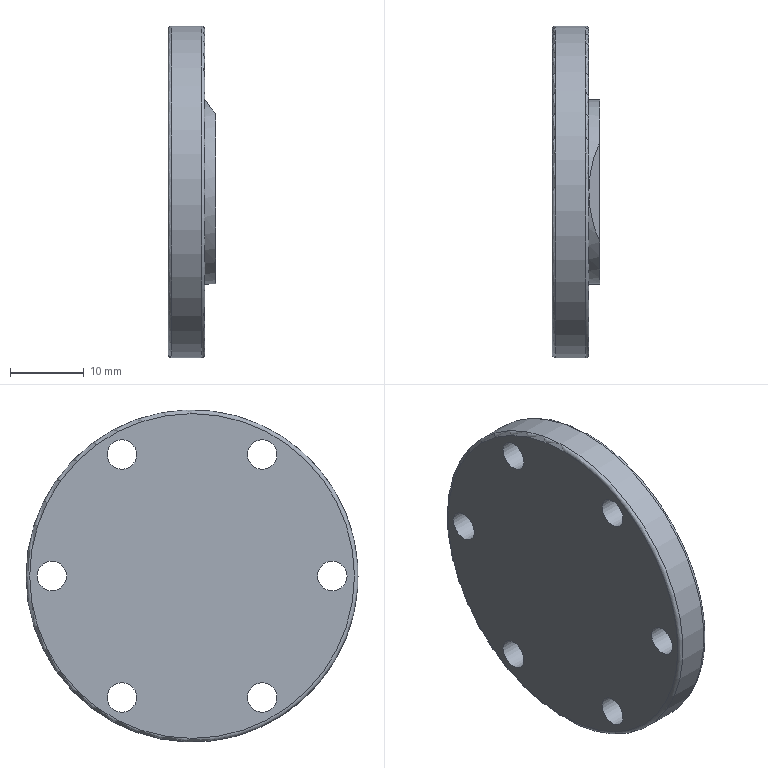Part | STEP file | 1-07 | 1 solid | 15 faces | box 6.5 x 45 x 45 mm | volume 8285 mm3 | cylinder 9 | plane 4 | torus 2 | commonest cylinder face diameters 4 x6 25 x2 45 x1
STEP:
#1=CARTESIAN_POINT('',(0.,0.,0.));
#2=DIRECTION('',(0.,0.,1.));
#3=DIRECTION('',(1.,0.,0.));
#4=AXIS2_PLACEMENT_3D('',#1,#2,#3);
#5=CARTESIAN_POINT('',(0.,21.,0.));
#6=VERTEX_POINT('',#5);
#7=CARTESIAN_POINT('',(0.,19.,0.));
#8=DIRECTION('',(-1.,0.,0.));
#9=DIRECTION('',(0.,1.,0.));
#10=AXIS2_PLACEMENT_3D('',#7,#8,#9);
#11=CIRCLE('',#10,2.);
#12=CARTESIAN_POINT('',(0.,19.,0.));
#13=DIRECTION('',(-1.,0.,0.));
#14=DIRECTION('',(0.,1.,0.));
#15=AXIS2_PLACEMENT_3D('',#12,#13,#14);
#16=CYLINDRICAL_SURFACE('',#15,2.);
#17=CARTESIAN_POINT('',(0.,0.));
#18=DIRECTION('',(1.,0.));
#19=VECTOR('',#18,1.);
#20=LINE('',#17,#19);
#21=(GEOMETRIC_REPRESENTATION_CONTEXT(2)PARAMETRIC_REPRESENTATION_CONTEXT()REPRESENTATION_CONTEXT('',''));
#22=DEFINITIONAL_REPRESENTATION('',(#20),#21);
#23=PCURVE('',#16,#22);
#24=CARTESIAN_POINT('',(0.,-6.029,0.));
#25=DIRECTION('',(1.,0.,0.));
#26=DIRECTION('',(0.,1.,0.));
#27=AXIS2_PLACEMENT_3D('',#24,#25,#26);
#28=PLANE('',#27);
#29=CARTESIAN_POINT('',(27.029,0.));
#30=CARTESIAN_POINT('',(27.029,-3.464));
#31=CARTESIAN_POINT('',(24.029,-1.732));
#32=CARTESIAN_POINT('',(21.029,0.));
#33=CARTESIAN_POINT('',(24.029,1.732));
#34=CARTESIAN_POINT('',(27.029,3.464));
#35=CARTESIAN_POINT('',(27.029,0.));
#36=(BOUNDED_CURVE()B_SPLINE_CURVE(2,(#29,#30,#31,#32,#33,#34,#35),.UNSPECIFIED.,.T.,.F.)B_SPLINE_CURVE_WITH_KNOTS((1,2,2,2,2,1),(-2.094,0.,2.094,4.189,6.283,8.378),.UNSPECIFIED.)CURVE()GEOMETRIC_REPRESENTATION_ITEM()RATIONAL_B_SPLINE_CURVE((1.,0.5,1.,0.5,1.,0.5,1.))REPRESENTATION_ITEM(''));
#37=(GEOMETRIC_REPRESENTATION_CONTEXT(2)PARAMETRIC_REPRESENTATION_CONTEXT()REPRESENTATION_CONTEXT('',''));
#38=DEFINITIONAL_REPRESENTATION('',(#36),#37);
#39=PCURVE('',#28,#38);
#40=SURFACE_CURVE('',#11,(#23,#39),.PCURVE_S1.);
#41=EDGE_CURVE('',#6,#6,#40,.T.);
#42=ORIENTED_EDGE('',*,*,#41,.T.);
#43=CARTESIAN_POINT('',(-5.,21.,0.));
#44=VERTEX_POINT('',#43);
#45=CARTESIAN_POINT('',(0.,21.,0.));
#46=DIRECTION('',(-1.,0.,0.));
#47=VECTOR('',#46,1.);
#48=LINE('',#45,#47);
#49=CARTESIAN_POINT('',(6.283,0.));
#50=DIRECTION('',(0.,1.));
#51=VECTOR('',#50,1.);
#52=LINE('',#49,#51);
#53=(GEOMETRIC_REPRESENTATION_CONTEXT(2)PARAMETRIC_REPRESENTATION_CONTEXT()REPRESENTATION_CONTEXT('',''));
#54=DEFINITIONAL_REPRESENTATION('',(#52),#53);
#55=PCURVE('',#16,#54);
#56=CARTESIAN_POINT('',(0.,0.));
#57=DIRECTION('',(0.,1.));
#58=VECTOR('',#57,1.);
#59=LINE('',#56,#58);
#60=(GEOMETRIC_REPRESENTATION_CONTEXT(2)PARAMETRIC_REPRESENTATION_CONTEXT()REPRESENTATION_CONTEXT('',''));
#61=DEFINITIONAL_REPRESENTATION('',(#59),#60);
#62=PCURVE('',#16,#61);
#63=SEAM_CURVE('',#48,(#55,#62),.PCURVE_S1.);
#64=EDGE_CURVE('',#6,#44,#63,.T.);
#65=ORIENTED_EDGE('',*,*,#64,.T.);
#66=CARTESIAN_POINT('',(-5.,19.,0.));
#67=DIRECTION('',(-1.,0.,0.));
#68=DIRECTION('',(0.,1.,0.));
#69=AXIS2_PLACEMENT_3D('',#66,#67,#68);
#70=CIRCLE('',#69,2.);
#71=CARTESIAN_POINT('',(0.,5.));
#72=DIRECTION('',(1.,0.));
#73=VECTOR('',#72,1.);
#74=LINE('',#71,#73);
#75=(GEOMETRIC_REPRESENTATION_CONTEXT(2)PARAMETRIC_REPRESENTATION_CONTEXT()REPRESENTATION_CONTEXT('',''));
#76=DEFINITIONAL_REPRESENTATION('',(#74),#75);
#77=PCURVE('',#16,#76);
#78=CARTESIAN_POINT('',(-5.,-6.029,0.));
#79=DIRECTION('',(1.,0.,0.));
#80=DIRECTION('',(0.,1.,0.));
#81=AXIS2_PLACEMENT_3D('',#78,#79,#80);
#82=PLANE('',#81);
#83=CARTESIAN_POINT('',(27.029,0.));
#84=CARTESIAN_POINT('',(27.029,-3.464));
#85=CARTESIAN_POINT('',(24.029,-1.732));
#86=CARTESIAN_POINT('',(21.029,0.));
#87=CARTESIAN_POINT('',(24.029,1.732));
#88=CARTESIAN_POINT('',(27.029,3.464));
#89=CARTESIAN_POINT('',(27.029,0.));
#90=(BOUNDED_CURVE()B_SPLINE_CURVE(2,(#83,#84,#85,#86,#87,#88,#89),.UNSPECIFIED.,.T.,.F.)B_SPLINE_CURVE_WITH_KNOTS((1,2,2,2,2,1),(-2.094,0.,2.094,4.189,6.283,8.378),.UNSPECIFIED.)CURVE()GEOMETRIC_REPRESENTATION_ITEM()RATIONAL_B_SPLINE_CURVE((1.,0.5,1.,0.5,1.,0.5,1.))REPRESENTATION_ITEM(''));
#91=(GEOMETRIC_REPRESENTATION_CONTEXT(2)PARAMETRIC_REPRESENTATION_CONTEXT()REPRESENTATION_CONTEXT('',''));
#92=DEFINITIONAL_REPRESENTATION('',(#90),#91);
#93=PCURVE('',#82,#92);
#94=SURFACE_CURVE('',#70,(#77,#93),.PCURVE_S1.);
#95=EDGE_CURVE('',#44,#44,#94,.T.);
#96=ORIENTED_EDGE('',*,*,#95,.F.);
#97=ORIENTED_EDGE('',*,*,#64,.F.);
#98=EDGE_LOOP('',(#42,#65,#96,#97));
#99=FACE_BOUND('',#98,.F.);
#100=ADVANCED_FACE('',(#99),#16,.F.);
#101=CARTESIAN_POINT('',(0.,11.5,16.454));
#102=VERTEX_POINT('',#101);
#103=CARTESIAN_POINT('',(0.,9.5,16.454));
#104=DIRECTION('',(-1.,0.,0.));
#105=DIRECTION('',(0.,1.,0.));
#106=AXIS2_PLACEMENT_3D('',#103,#104,#105);
#107=CIRCLE('',#106,2.);
#108=CARTESIAN_POINT('',(0.,9.5,16.454));
#109=DIRECTION('',(-1.,0.,0.));
#110=DIRECTION('',(0.,1.,0.));
#111=AXIS2_PLACEMENT_3D('',#108,#109,#110);
#112=CYLINDRICAL_SURFACE('',#111,2.);
#113=CARTESIAN_POINT('',(0.,0.));
#114=DIRECTION('',(1.,0.));
#115=VECTOR('',#114,1.);
#116=LINE('',#113,#115);
#117=(GEOMETRIC_REPRESENTATION_CONTEXT(2)PARAMETRIC_REPRESENTATION_CONTEXT()REPRESENTATION_CONTEXT('',''));
#118=DEFINITIONAL_REPRESENTATION('',(#116),#117);
#119=PCURVE('',#112,#118);
#120=CARTESIAN_POINT('',(17.529,16.454));
#121=CARTESIAN_POINT('',(17.529,12.99));
#122=CARTESIAN_POINT('',(14.529,14.722));
#123=CARTESIAN_POINT('',(11.529,16.454));
#124=CARTESIAN_POINT('',(14.529,18.187));
#125=CARTESIAN_POINT('',(17.529,19.919));
#126=CARTESIAN_POINT('',(17.529,16.454));
#127=(BOUNDED_CURVE()B_SPLINE_CURVE(2,(#120,#121,#122,#123,#124,#125,#126),.UNSPECIFIED.,.T.,.F.)B_SPLINE_CURVE_WITH_KNOTS((1,2,2,2,2,1),(-2.094,0.,2.094,4.189,6.283,8.378),.UNSPECIFIED.)CURVE()GEOMETRIC_REPRESENTATION_ITEM()RATIONAL_B_SPLINE_CURVE((1.,0.5,1.,0.5,1.,0.5,1.))REPRESENTATION_ITEM(''));
#128=(GEOMETRIC_REPRESENTATION_CONTEXT(2)PARAMETRIC_REPRESENTATION_CONTEXT()REPRESENTATION_CONTEXT('',''));
#129=DEFINITIONAL_REPRESENTATION('',(#127),#128);
#130=PCURVE('',#28,#129);
#131=SURFACE_CURVE('',#107,(#119,#130),.PCURVE_S1.);
#132=EDGE_CURVE('',#102,#102,#131,.T.);
#133=ORIENTED_EDGE('',*,*,#132,.T.);
#134=CARTESIAN_POINT('',(-5.,11.5,16.454));
#135=VERTEX_POINT('',#134);
#136=CARTESIAN_POINT('',(0.,11.5,16.454));
#137=DIRECTION('',(-1.,0.,0.));
#138=VECTOR('',#137,1.);
#139=LINE('',#136,#138);
#140=CARTESIAN_POINT('',(6.283,0.));
#141=DIRECTION('',(0.,1.));
#142=VECTOR('',#141,1.);
#143=LINE('',#140,#142);
#144=(GEOMETRIC_REPRESENTATION_CONTEXT(2)PARAMETRIC_REPRESENTATION_CONTEXT()REPRESENTATION_CONTEXT('',''));
#145=DEFINITIONAL_REPRESENTATION('',(#143),#144);
#146=PCURVE('',#112,#145);
#147=CARTESIAN_POINT('',(0.,0.));
#148=DIRECTION('',(0.,1.));
#149=VECTOR('',#148,1.);
#150=LINE('',#147,#149);
#151=(GEOMETRIC_REPRESENTATION_CONTEXT(2)PARAMETRIC_REPRESENTATION_CONTEXT()REPRESENTATION_CONTEXT('',''));
#152=DEFINITIONAL_REPRESENTATION('',(#150),#151);
#153=PCURVE('',#112,#152);
#154=SEAM_CURVE('',#139,(#146,#153),.PCURVE_S1.);
#155=EDGE_CURVE('',#102,#135,#154,.T.);
#156=ORIENTED_EDGE('',*,*,#155,.T.);
#157=CARTESIAN_POINT('',(-5.,9.5,16.454));
#158=DIRECTION('',(-1.,0.,0.));
#159=DIRECTION('',(0.,1.,0.));
#160=AXIS2_PLACEMENT_3D('',#157,#158,#159);
#161=CIRCLE('',#160,2.);
#162=CARTESIAN_POINT('',(0.,5.));
#163=DIRECTION('',(1.,0.));
#164=VECTOR('',#163,1.);
#165=LINE('',#162,#164);
#166=(GEOMETRIC_REPRESENTATION_CONTEXT(2)PARAMETRIC_REPRESENTATION_CONTEXT()REPRESENTATION_CONTEXT('',''));
#167=DEFINITIONAL_REPRESENTATION('',(#165),#166);
#168=PCURVE('',#112,#167);
#169=CARTESIAN_POINT('',(17.529,16.454));
#170=CARTESIAN_POINT('',(17.529,12.99));
#171=CARTESIAN_POINT('',(14.529,14.722));
#172=CARTESIAN_POINT('',(11.529,16.454));
#173=CARTESIAN_POINT('',(14.529,18.187));
#174=CARTESIAN_POINT('',(17.529,19.919));
#175=CARTESIAN_POINT('',(17.529,16.454));
#176=(BOUNDED_CURVE()B_SPLINE_CURVE(2,(#169,#170,#171,#172,#173,#174,#175),.UNSPECIFIED.,.T.,.F.)B_SPLINE_CURVE_WITH_KNOTS((1,2,2,2,2,1),(-2.094,0.,2.094,4.189,6.283,8.378),.UNSPECIFIED.)CURVE()GEOMETRIC_REPRESENTATION_ITEM()RATIONAL_B_SPLINE_CURVE((1.,0.5,1.,0.5,1.,0.5,1.))REPRESENTATION_ITEM(''));
#177=(GEOMETRIC_REPRESENTATION_CONTEXT(2)PARAMETRIC_REPRESENTATION_CONTEXT()REPRESENTATION_CONTEXT('',''));
#178=DEFINITIONAL_REPRESENTATION('',(#176),#177);
#179=PCURVE('',#82,#178);
#180=SURFACE_CURVE('',#161,(#168,#179),.PCURVE_S1.);
#181=EDGE_CURVE('',#135,#135,#180,.T.);
#182=ORIENTED_EDGE('',*,*,#181,.F.);
#183=ORIENTED_EDGE('',*,*,#155,.F.);
#184=EDGE_LOOP('',(#133,#156,#182,#183));
#185=FACE_BOUND('',#184,.F.);
#186=ADVANCED_FACE('',(#185),#112,.F.);
#187=CARTESIAN_POINT('',(0.,-7.5,16.454));
#188=VERTEX_POINT('',#187);
#189=CARTESIAN_POINT('',(0.,-9.5,16.454));
#190=DIRECTION('',(-1.,0.,0.));
#191=DIRECTION('',(0.,1.,0.));
#192=AXIS2_PLACEMENT_3D('',#189,#190,#191);
#193=CIRCLE('',#192,2.);
#194=CARTESIAN_POINT('',(0.,-9.5,16.454));
#195=DIRECTION('',(-1.,0.,0.));
#196=DIRECTION('',(0.,1.,0.));
#197=AXIS2_PLACEMENT_3D('',#194,#195,#196);
#198=CYLINDRICAL_SURFACE('',#197,2.);
#199=CARTESIAN_POINT('',(0.,0.));
#200=DIRECTION('',(1.,0.));
#201=VECTOR('',#200,1.);
#202=LINE('',#199,#201);
#203=(GEOMETRIC_REPRESENTATION_CONTEXT(2)PARAMETRIC_REPRESENTATION_CONTEXT()REPRESENTATION_CONTEXT('',''));
#204=DEFINITIONAL_REPRESENTATION('',(#202),#203);
#205=PCURVE('',#198,#204);
#206=CARTESIAN_POINT('',(-1.471,16.454));
#207=CARTESIAN_POINT('',(-1.471,12.99));
#208=CARTESIAN_POINT('',(-4.471,14.722));
#209=CARTESIAN_POINT('',(-7.471,16.454));
#210=CARTESIAN_POINT('',(-4.471,18.187));
#211=CARTESIAN_POINT('',(-1.471,19.919));
#212=CARTESIAN_POINT('',(-1.471,16.454));
#213=(BOUNDED_CURVE()B_SPLINE_CURVE(2,(#206,#207,#208,#209,#210,#211,#212),.UNSPECIFIED.,.T.,.F.)B_SPLINE_CURVE_WITH_KNOTS((1,2,2,2,2,1),(-2.094,0.,2.094,4.189,6.283,8.378),.UNSPECIFIED.)CURVE()GEOMETRIC_REPRESENTATION_ITEM()RATIONAL_B_SPLINE_CURVE((1.,0.5,1.,0.5,1.,0.5,1.))REPRESENTATION_ITEM(''));
#214=(GEOMETRIC_REPRESENTATION_CONTEXT(2)PARAMETRIC_REPRESENTATION_CONTEXT()REPRESENTATION_CONTEXT('',''));
#215=DEFINITIONAL_REPRESENTATION('',(#213),#214);
#216=PCURVE('',#28,#215);
#217=SURFACE_CURVE('',#193,(#205,#216),.PCURVE_S1.);
#218=EDGE_CURVE('',#188,#188,#217,.T.);
#219=ORIENTED_EDGE('',*,*,#218,.T.);
#220=CARTESIAN_POINT('',(-5.,-7.5,16.454));
#221=VERTEX_POINT('',#220);
#222=CARTESIAN_POINT('',(0.,-7.5,16.454));
#223=DIRECTION('',(-1.,0.,0.));
#224=VECTOR('',#223,1.);
#225=LINE('',#222,#224);
#226=CARTESIAN_POINT('',(6.283,0.));
#227=DIRECTION('',(0.,1.));
#228=VECTOR('',#227,1.);
#229=LINE('',#226,#228);
#230=(GEOMETRIC_REPRESENTATION_CONTEXT(2)PARAMETRIC_REPRESENTATION_CONTEXT()REPRESENTATION_CONTEXT('',''));
#231=DEFINITIONAL_REPRESENTATION('',(#229),#230);
#232=PCURVE('',#198,#231);
#233=CARTESIAN_POINT('',(0.,0.));
#234=DIRECTION('',(0.,1.));
#235=VECTOR('',#234,1.);
#236=LINE('',#233,#235);
#237=(GEOMETRIC_REPRESENTATION_CONTEXT(2)PARAMETRIC_REPRESENTATION_CONTEXT()REPRESENTATION_CONTEXT('',''));
#238=DEFINITIONAL_REPRESENTATION('',(#236),#237);
#239=PCURVE('',#198,#238);
#240=SEAM_CURVE('',#225,(#232,#239),.PCURVE_S1.);
#241=EDGE_CURVE('',#188,#221,#240,.T.);
#242=ORIENTED_EDGE('',*,*,#241,.T.);
#243=CARTESIAN_POINT('',(-5.,-9.5,16.454));
#244=DIRECTION('',(-1.,0.,0.));
#245=DIRECTION('',(0.,1.,0.));
#246=AXIS2_PLACEMENT_3D('',#243,#244,#245);
#247=CIRCLE('',#246,2.);
#248=CARTESIAN_POINT('',(0.,5.));
#249=DIRECTION('',(1.,0.));
#250=VECTOR('',#249,1.);
#251=LINE('',#248,#250);
#252=(GEOMETRIC_REPRESENTATION_CONTEXT(2)PARAMETRIC_REPRESENTATION_CONTEXT()REPRESENTATION_CONTEXT('',''));
#253=DEFINITIONAL_REPRESENTATION('',(#251),#252);
#254=PCURVE('',#198,#253);
#255=CARTESIAN_POINT('',(-1.471,16.454));
#256=CARTESIAN_POINT('',(-1.471,12.99));
#257=CARTESIAN_POINT('',(-4.471,14.722));
#258=CARTESIAN_POINT('',(-7.471,16.454));
#259=CARTESIAN_POINT('',(-4.471,18.187));
#260=CARTESIAN_POINT('',(-1.471,19.919));
#261=CARTESIAN_POINT('',(-1.471,16.454));
#262=(BOUNDED_CURVE()B_SPLINE_CURVE(2,(#255,#256,#257,#258,#259,#260,#261),.UNSPECIFIED.,.T.,.F.)B_SPLINE_CURVE_WITH_KNOTS((1,2,2,2,2,1),(-2.094,0.,2.094,4.189,6.283,8.378),.UNSPECIFIED.)CURVE()GEOMETRIC_REPRESENTATION_ITEM()RATIONAL_B_SPLINE_CURVE((1.,0.5,1.,0.5,1.,0.5,1.))REPRESENTATION_ITEM(''));
#263=(GEOMETRIC_REPRESENTATION_CONTEXT(2)PARAMETRIC_REPRESENTATION_CONTEXT()REPRESENTATION_CONTEXT('',''));
#264=DEFINITIONAL_REPRESENTATION('',(#262),#263);
#265=PCURVE('',#82,#264);
#266=SURFACE_CURVE('',#247,(#254,#265),.PCURVE_S1.);
#267=EDGE_CURVE('',#221,#221,#266,.T.);
#268=ORIENTED_EDGE('',*,*,#267,.F.);
#269=ORIENTED_EDGE('',*,*,#241,.F.);
#270=EDGE_LOOP('',(#219,#242,#268,#269));
#271=FACE_BOUND('',#270,.F.);
#272=ADVANCED_FACE('',(#271),#198,.F.);
#273=CARTESIAN_POINT('',(0.,-17.,0.));
#274=VERTEX_POINT('',#273);
#275=CARTESIAN_POINT('',(0.,-19.,0.));
#276=DIRECTION('',(-1.,0.,0.));
#277=DIRECTION('',(0.,1.,0.));
#278=AXIS2_PLACEMENT_3D('',#275,#276,#277);
#279=CIRCLE('',#278,2.);
#280=CARTESIAN_POINT('',(0.,-19.,0.));
#281=DIRECTION('',(-1.,0.,0.));
#282=DIRECTION('',(0.,1.,0.));
#283=AXIS2_PLACEMENT_3D('',#280,#281,#282);
#284=CYLINDRICAL_SURFACE('',#283,2.);
#285=CARTESIAN_POINT('',(0.,0.));
#286=DIRECTION('',(1.,0.));
#287=VECTOR('',#286,1.);
#288=LINE('',#285,#287);
#289=(GEOMETRIC_REPRESENTATION_CONTEXT(2)PARAMETRIC_REPRESENTATION_CONTEXT()REPRESENTATION_CONTEXT('',''));
#290=DEFINITIONAL_REPRESENTATION('',(#288),#289);
#291=PCURVE('',#284,#290);
#292=CARTESIAN_POINT('',(-10.971,0.));
#293=CARTESIAN_POINT('',(-10.971,-3.464));
#294=CARTESIAN_POINT('',(-13.971,-1.732));
#295=CARTESIAN_POINT('',(-16.971,0.));
#296=CARTESIAN_POINT('',(-13.971,1.732));
#297=CARTESIAN_POINT('',(-10.971,3.464));
#298=CARTESIAN_POINT('',(-10.971,0.));
#299=(BOUNDED_CURVE()B_SPLINE_CURVE(2,(#292,#293,#294,#295,#296,#297,#298),.UNSPECIFIED.,.T.,.F.)B_SPLINE_CURVE_WITH_KNOTS((1,2,2,2,2,1),(-2.094,0.,2.094,4.189,6.283,8.378),.UNSPECIFIED.)CURVE()GEOMETRIC_REPRESENTATION_ITEM()RATIONAL_B_SPLINE_CURVE((1.,0.5,1.,0.5,1.,0.5,1.))REPRESENTATION_ITEM(''));
#300=(GEOMETRIC_REPRESENTATION_CONTEXT(2)PARAMETRIC_REPRESENTATION_CONTEXT()REPRESENTATION_CONTEXT('',''));
#301=DEFINITIONAL_REPRESENTATION('',(#299),#300);
#302=PCURVE('',#28,#301);
#303=SURFACE_CURVE('',#279,(#291,#302),.PCURVE_S1.);
#304=EDGE_CURVE('',#274,#274,#303,.T.);
#305=ORIENTED_EDGE('',*,*,#304,.T.);
#306=CARTESIAN_POINT('',(-5.,-17.,0.));
#307=VERTEX_POINT('',#306);
#308=CARTESIAN_POINT('',(0.,-17.,0.));
#309=DIRECTION('',(-1.,0.,0.));
#310=VECTOR('',#309,1.);
#311=LINE('',#308,#310);
#312=CARTESIAN_POINT('',(6.283,0.));
#313=DIRECTION('',(0.,1.));
#314=VECTOR('',#313,1.);
#315=LINE('',#312,#314);
#316=(GEOMETRIC_REPRESENTATION_CONTEXT(2)PARAMETRIC_REPRESENTATION_CONTEXT()REPRESENTATION_CONTEXT('',''));
#317=DEFINITIONAL_REPRESENTATION('',(#315),#316);
#318=PCURVE('',#284,#317);
#319=CARTESIAN_POINT('',(0.,0.));
#320=DIRECTION('',(0.,1.));
#321=VECTOR('',#320,1.);
#322=LINE('',#319,#321);
#323=(GEOMETRIC_REPRESENTATION_CONTEXT(2)PARAMETRIC_REPRESENTATION_CONTEXT()REPRESENTATION_CONTEXT('',''));
#324=DEFINITIONAL_REPRESENTATION('',(#322),#323);
#325=PCURVE('',#284,#324);
#326=SEAM_CURVE('',#311,(#318,#325),.PCURVE_S1.);
#327=EDGE_CURVE('',#274,#307,#326,.T.);
#328=ORIENTED_EDGE('',*,*,#327,.T.);
#329=CARTESIAN_POINT('',(-5.,-19.,0.));
#330=DIRECTION('',(-1.,0.,0.));
#331=DIRECTION('',(0.,1.,0.));
#332=AXIS2_PLACEMENT_3D('',#329,#330,#331);
#333=CIRCLE('',#332,2.);
#334=CARTESIAN_POINT('',(0.,5.));
#335=DIRECTION('',(1.,0.));
#336=VECTOR('',#335,1.);
#337=LINE('',#334,#336);
#338=(GEOMETRIC_REPRESENTATION_CONTEXT(2)PARAMETRIC_REPRESENTATION_CONTEXT()REPRESENTATION_CONTEXT('',''));
#339=DEFINITIONAL_REPRESENTATION('',(#337),#338);
#340=PCURVE('',#284,#339);
#341=CARTESIAN_POINT('',(-10.971,0.));
#342=CARTESIAN_POINT('',(-10.971,-3.464));
#343=CARTESIAN_POINT('',(-13.971,-1.732));
#344=CARTESIAN_POINT('',(-16.971,0.));
#345=CARTESIAN_POINT('',(-13.971,1.732));
#346=CARTESIAN_POINT('',(-10.971,3.464));
#347=CARTESIAN_POINT('',(-10.971,0.));
#348=(BOUNDED_CURVE()B_SPLINE_CURVE(2,(#341,#342,#343,#344,#345,#346,#347),.UNSPECIFIED.,.T.,.F.)B_SPLINE_CURVE_WITH_KNOTS((1,2,2,2,2,1),(-2.094,0.,2.094,4.189,6.283,8.378),.UNSPECIFIED.)CURVE()GEOMETRIC_REPRESENTATION_ITEM()RATIONAL_B_SPLINE_CURVE((1.,0.5,1.,0.5,1.,0.5,1.))REPRESENTATION_ITEM(''));
#349=(GEOMETRIC_REPRESENTATION_CONTEXT(2)PARAMETRIC_REPRESENTATION_CONTEXT()REPRESENTATION_CONTEXT('',''));
#350=DEFINITIONAL_REPRESENTATION('',(#348),#349);
#351=PCURVE('',#82,#350);
#352=SURFACE_CURVE('',#333,(#340,#351),.PCURVE_S1.);
#353=EDGE_CURVE('',#307,#307,#352,.T.);
#354=ORIENTED_EDGE('',*,*,#353,.F.);
#355=ORIENTED_EDGE('',*,*,#327,.F.);
#356=EDGE_LOOP('',(#305,#328,#354,#355));
#357=FACE_BOUND('',#356,.F.);
#358=ADVANCED_FACE('',(#357),#284,.F.);
#359=CARTESIAN_POINT('',(0.,-7.5,-16.454));
#360=VERTEX_POINT('',#359);
#361=CARTESIAN_POINT('',(0.,-9.5,-16.454));
#362=DIRECTION('',(-1.,0.,0.));
#363=DIRECTION('',(0.,1.,0.));
#364=AXIS2_PLACEMENT_3D('',#361,#362,#363);
#365=CIRCLE('',#364,2.);
#366=CARTESIAN_POINT('',(0.,-9.5,-16.454));
#367=DIRECTION('',(-1.,0.,0.));
#368=DIRECTION('',(0.,1.,0.));
#369=AXIS2_PLACEMENT_3D('',#366,#367,#368);
#370=CYLINDRICAL_SURFACE('',#369,2.);
#371=CARTESIAN_POINT('',(0.,0.));
#372=DIRECTION('',(1.,0.));
#373=VECTOR('',#372,1.);
#374=LINE('',#371,#373);
#375=(GEOMETRIC_REPRESENTATION_CONTEXT(2)PARAMETRIC_REPRESENTATION_CONTEXT()REPRESENTATION_CONTEXT('',''));
#376=DEFINITIONAL_REPRESENTATION('',(#374),#375);
#377=PCURVE('',#370,#376);
#378=CARTESIAN_POINT('',(-1.471,-16.454));
#379=CARTESIAN_POINT('',(-1.471,-19.919));
#380=CARTESIAN_POINT('',(-4.471,-18.187));
#381=CARTESIAN_POINT('',(-7.471,-16.454));
#382=CARTESIAN_POINT('',(-4.471,-14.722));
#383=CARTESIAN_POINT('',(-1.471,-12.99));
#384=CARTESIAN_POINT('',(-1.471,-16.454));
#385=(BOUNDED_CURVE()B_SPLINE_CURVE(2,(#378,#379,#380,#381,#382,#383,#384),.UNSPECIFIED.,.T.,.F.)B_SPLINE_CURVE_WITH_KNOTS((1,2,2,2,2,1),(-2.094,0.,2.094,4.189,6.283,8.378),.UNSPECIFIED.)CURVE()GEOMETRIC_REPRESENTATION_ITEM()RATIONAL_B_SPLINE_CURVE((1.,0.5,1.,0.5,1.,0.5,1.))REPRESENTATION_ITEM(''));
#386=(GEOMETRIC_REPRESENTATION_CONTEXT(2)PARAMETRIC_REPRESENTATION_CONTEXT()REPRESENTATION_CONTEXT('',''));
#387=DEFINITIONAL_REPRESENTATION('',(#385),#386);
#388=PCURVE('',#28,#387);
#389=SURFACE_CURVE('',#365,(#377,#388),.PCURVE_S1.);
#390=EDGE_CURVE('',#360,#360,#389,.T.);
#391=ORIENTED_EDGE('',*,*,#390,.T.);
#392=CARTESIAN_POINT('',(-5.,-7.5,-16.454));
#393=VERTEX_POINT('',#392);
#394=CARTESIAN_POINT('',(0.,-7.5,-16.454));
#395=DIRECTION('',(-1.,0.,0.));
#396=VECTOR('',#395,1.);
#397=LINE('',#394,#396);
#398=CARTESIAN_POINT('',(6.283,0.));
#399=DIRECTION('',(0.,1.));
#400=VECTOR('',#399,1.);
#401=LINE('',#398,#400);
#402=(GEOMETRIC_REPRESENTATION_CONTEXT(2)PARAMETRIC_REPRESENTATION_CONTEXT()REPRESENTATION_CONTEXT('',''));
#403=DEFINITIONAL_REPRESENTATION('',(#401),#402);
#404=PCURVE('',#370,#403);
#405=CARTESIAN_POINT('',(0.,0.));
#406=DIRECTION('',(0.,1.));
#407=VECTOR('',#406,1.);
#408=LINE('',#405,#407);
#409=(GEOMETRIC_REPRESENTATION_CONTEXT(2)PARAMETRIC_REPRESENTATION_CONTEXT()REPRESENTATION_CONTEXT('',''));
#410=DEFINITIONAL_REPRESENTATION('',(#408),#409);
#411=PCURVE('',#370,#410);
#412=SEAM_CURVE('',#397,(#404,#411),.PCURVE_S1.);
#413=EDGE_CURVE('',#360,#393,#412,.T.);
#414=ORIENTED_EDGE('',*,*,#413,.T.);
#415=CARTESIAN_POINT('',(-5.,-9.5,-16.454));
#416=DIRECTION('',(-1.,0.,0.));
#417=DIRECTION('',(0.,1.,0.));
#418=AXIS2_PLACEMENT_3D('',#415,#416,#417);
#419=CIRCLE('',#418,2.);
#420=CARTESIAN_POINT('',(0.,5.));
#421=DIRECTION('',(1.,0.));
#422=VECTOR('',#421,1.);
#423=LINE('',#420,#422);
#424=(GEOMETRIC_REPRESENTATION_CONTEXT(2)PARAMETRIC_REPRESENTATION_CONTEXT()REPRESENTATION_CONTEXT('',''));
#425=DEFINITIONAL_REPRESENTATION('',(#423),#424);
#426=PCURVE('',#370,#425);
#427=CARTESIAN_POINT('',(-1.471,-16.454));
#428=CARTESIAN_POINT('',(-1.471,-19.919));
#429=CARTESIAN_POINT('',(-4.471,-18.187));
#430=CARTESIAN_POINT('',(-7.471,-16.454));
#431=CARTESIAN_POINT('',(-4.471,-14.722));
#432=CARTESIAN_POINT('',(-1.471,-12.99));
#433=CARTESIAN_POINT('',(-1.471,-16.454));
#434=(BOUNDED_CURVE()B_SPLINE_CURVE(2,(#427,#428,#429,#430,#431,#432,#433),.UNSPECIFIED.,.T.,.F.)B_SPLINE_CURVE_WITH_KNOTS((1,2,2,2,2,1),(-2.094,0.,2.094,4.189,6.283,8.378),.UNSPECIFIED.)CURVE()GEOMETRIC_REPRESENTATION_ITEM()RATIONAL_B_SPLINE_CURVE((1.,0.5,1.,0.5,1.,0.5,1.))REPRESENTATION_ITEM(''));
#435=(GEOMETRIC_REPRESENTATION_CONTEXT(2)PARAMETRIC_REPRESENTATION_CONTEXT()REPRESENTATION_CONTEXT('',''));
#436=DEFINITIONAL_REPRESENTATION('',(#434),#435);
#437=PCURVE('',#82,#436);
#438=SURFACE_CURVE('',#419,(#426,#437),.PCURVE_S1.);
#439=EDGE_CURVE('',#393,#393,#438,.T.);
#440=ORIENTED_EDGE('',*,*,#439,.F.);
#441=ORIENTED_EDGE('',*,*,#413,.F.);
#442=EDGE_LOOP('',(#391,#414,#440,#441));
#443=FACE_BOUND('',#442,.F.);
#444=ADVANCED_FACE('',(#443),#370,.F.);
#445=CARTESIAN_POINT('',(0.,11.5,-16.454));
#446=VERTEX_POINT('',#445);
#447=CARTESIAN_POINT('',(0.,9.5,-16.454));
#448=DIRECTION('',(-1.,0.,0.));
#449=DIRECTION('',(0.,1.,0.));
#450=AXIS2_PLACEMENT_3D('',#447,#448,#449);
#451=CIRCLE('',#450,2.);
#452=CARTESIAN_POINT('',(0.,9.5,-16.454));
#453=DIRECTION('',(-1.,0.,0.));
#454=DIRECTION('',(0.,1.,0.));
#455=AXIS2_PLACEMENT_3D('',#452,#453,#454);
#456=CYLINDRICAL_SURFACE('',#455,2.);
#457=CARTESIAN_POINT('',(0.,0.));
#458=DIRECTION('',(1.,0.));
#459=VECTOR('',#458,1.);
#460=LINE('',#457,#459);
#461=(GEOMETRIC_REPRESENTATION_CONTEXT(2)PARAMETRIC_REPRESENTATION_CONTEXT()REPRESENTATION_CONTEXT('',''));
#462=DEFINITIONAL_REPRESENTATION('',(#460),#461);
#463=PCURVE('',#456,#462);
#464=CARTESIAN_POINT('',(17.529,-16.454));
#465=CARTESIAN_POINT('',(17.529,-19.919));
#466=CARTESIAN_POINT('',(14.529,-18.187));
#467=CARTESIAN_POINT('',(11.529,-16.454));
#468=CARTESIAN_POINT('',(14.529,-14.722));
#469=CARTESIAN_POINT('',(17.529,-12.99));
#470=CARTESIAN_POINT('',(17.529,-16.454));
#471=(BOUNDED_CURVE()B_SPLINE_CURVE(2,(#464,#465,#466,#467,#468,#469,#470),.UNSPECIFIED.,.T.,.F.)B_SPLINE_CURVE_WITH_KNOTS((1,2,2,2,2,1),(-2.094,0.,2.094,4.189,6.283,8.378),.UNSPECIFIED.)CURVE()GEOMETRIC_REPRESENTATION_ITEM()RATIONAL_B_SPLINE_CURVE((1.,0.5,1.,0.5,1.,0.5,1.))REPRESENTATION_ITEM(''));
#472=(GEOMETRIC_REPRESENTATION_CONTEXT(2)PARAMETRIC_REPRESENTATION_CONTEXT()REPRESENTATION_CONTEXT('',''));
#473=DEFINITIONAL_REPRESENTATION('',(#471),#472);
#474=PCURVE('',#28,#473);
#475=SURFACE_CURVE('',#451,(#463,#474),.PCURVE_S1.);
#476=EDGE_CURVE('',#446,#446,#475,.T.);
#477=ORIENTED_EDGE('',*,*,#476,.T.);
#478=CARTESIAN_POINT('',(-5.,11.5,-16.454));
#479=VERTEX_POINT('',#478);
#480=CARTESIAN_POINT('',(0.,11.5,-16.454));
#481=DIRECTION('',(-1.,0.,0.));
#482=VECTOR('',#481,1.);
#483=LINE('',#480,#482);
#484=CARTESIAN_POINT('',(6.283,0.));
#485=DIRECTION('',(0.,1.));
#486=VECTOR('',#485,1.);
#487=LINE('',#484,#486);
#488=(GEOMETRIC_REPRESENTATION_CONTEXT(2)PARAMETRIC_REPRESENTATION_CONTEXT()REPRESENTATION_CONTEXT('',''));
#489=DEFINITIONAL_REPRESENTATION('',(#487),#488);
#490=PCURVE('',#456,#489);
#491=CARTESIAN_POINT('',(0.,0.));
#492=DIRECTION('',(0.,1.));
#493=VECTOR('',#492,1.);
#494=LINE('',#491,#493);
#495=(GEOMETRIC_REPRESENTATION_CONTEXT(2)PARAMETRIC_REPRESENTATION_CONTEXT()REPRESENTATION_CONTEXT('',''));
#496=DEFINITIONAL_REPRESENTATION('',(#494),#495);
#497=PCURVE('',#456,#496);
#498=SEAM_CURVE('',#483,(#490,#497),.PCURVE_S1.);
#499=EDGE_CURVE('',#446,#479,#498,.T.);
#500=ORIENTED_EDGE('',*,*,#499,.T.);
#501=CARTESIAN_POINT('',(-5.,9.5,-16.454));
#502=DIRECTION('',(-1.,0.,0.));
#503=DIRECTION('',(0.,1.,0.));
#504=AXIS2_PLACEMENT_3D('',#501,#502,#503);
#505=CIRCLE('',#504,2.);
#506=CARTESIAN_POINT('',(0.,5.));
#507=DIRECTION('',(1.,0.));
#508=VECTOR('',#507,1.);
#509=LINE('',#506,#508);
#510=(GEOMETRIC_REPRESENTATION_CONTEXT(2)PARAMETRIC_REPRESENTATION_CONTEXT()REPRESENTATION_CONTEXT('',''));
#511=DEFINITIONAL_REPRESENTATION('',(#509),#510);
#512=PCURVE('',#456,#511);
#513=CARTESIAN_POINT('',(17.529,-16.454));
#514=CARTESIAN_POINT('',(17.529,-19.919));
#515=CARTESIAN_POINT('',(14.529,-18.187));
#516=CARTESIAN_POINT('',(11.529,-16.454));
#517=CARTESIAN_POINT('',(14.529,-14.722));
#518=CARTESIAN_POINT('',(17.529,-12.99));
#519=CARTESIAN_POINT('',(17.529,-16.454));
#520=(BOUNDED_CURVE()B_SPLINE_CURVE(2,(#513,#514,#515,#516,#517,#518,#519),.UNSPECIFIED.,.T.,.F.)B_SPLINE_CURVE_WITH_KNOTS((1,2,2,2,2,1),(-2.094,0.,2.094,4.189,6.283,8.378),.UNSPECIFIED.)CURVE()GEOMETRIC_REPRESENTATION_ITEM()RATIONAL_B_SPLINE_CURVE((1.,0.5,1.,0.5,1.,0.5,1.))REPRESENTATION_ITEM(''));
#521=(GEOMETRIC_REPRESENTATION_CONTEXT(2)PARAMETRIC_REPRESENTATION_CONTEXT()REPRESENTATION_CONTEXT('',''));
#522=DEFINITIONAL_REPRESENTATION('',(#520),#521);
#523=PCURVE('',#82,#522);
#524=SURFACE_CURVE('',#505,(#512,#523),.PCURVE_S1.);
#525=EDGE_CURVE('',#479,#479,#524,.T.);
#526=ORIENTED_EDGE('',*,*,#525,.F.);
#527=ORIENTED_EDGE('',*,*,#499,.F.);
#528=EDGE_LOOP('',(#477,#500,#526,#527));
#529=FACE_BOUND('',#528,.F.);
#530=ADVANCED_FACE('',(#529),#456,.F.);
#531=CARTESIAN_POINT('',(1.5,-6.782,10.5));
#532=VERTEX_POINT('',#531);
#533=CARTESIAN_POINT('',(1.5,12.5,0.));
#534=VERTEX_POINT('',#533);
#535=CARTESIAN_POINT('',(1.5,0.,0.));
#536=DIRECTION('',(1.,0.,0.));
#537=DIRECTION('',(0.,-0.5426,0.84));
#538=AXIS2_PLACEMENT_3D('',#535,#536,#537);
#539=CIRCLE('',#538,12.5);
#540=CARTESIAN_POINT('',(0.,0.,0.));
#541=DIRECTION('',(1.,0.,0.));
#542=DIRECTION('',(0.,1.,0.));
#543=AXIS2_PLACEMENT_3D('',#540,#541,#542);
#544=CYLINDRICAL_SURFACE('',#543,12.5);
#545=CARTESIAN_POINT('',(2.144,1.5));
#546=DIRECTION('',(1.,0.));
#547=VECTOR('',#546,1.);
#548=LINE('',#545,#547);
#549=(GEOMETRIC_REPRESENTATION_CONTEXT(2)PARAMETRIC_REPRESENTATION_CONTEXT()REPRESENTATION_CONTEXT('',''));
#550=DEFINITIONAL_REPRESENTATION('',(#548),#549);
#551=PCURVE('',#544,#550);
#552=CARTESIAN_POINT('',(1.5,-3.349,0.));
#553=DIRECTION('',(1.,0.,0.));
#554=DIRECTION('',(0.,1.,0.));
#555=AXIS2_PLACEMENT_3D('',#552,#553,#554);
#556=PLANE('',#555);
#557=CARTESIAN_POINT('',(3.349,0.));
#558=DIRECTION('',(-0.5426,0.84));
#559=AXIS2_PLACEMENT_2D('',#557,#558);
#560=CIRCLE('',#559,12.5);
#561=(GEOMETRIC_REPRESENTATION_CONTEXT(2)PARAMETRIC_REPRESENTATION_CONTEXT()REPRESENTATION_CONTEXT('',''));
#562=DEFINITIONAL_REPRESENTATION('',(#560),#561);
#563=PCURVE('',#556,#562);
#564=SURFACE_CURVE('',#539,(#551,#563),.PCURVE_S1.);
#565=EDGE_CURVE('',#532,#534,#564,.T.);
#566=ORIENTED_EDGE('',*,*,#565,.F.);
#567=CARTESIAN_POINT('',(0.,0.,12.5));
#568=VERTEX_POINT('',#567);
#569=CARTESIAN_POINT('',(9.375,0.,0.));
#570=DIRECTION('',(0.8,0.,0.6));
#571=DIRECTION('',(-0.6,0.,0.8));
#572=AXIS2_PLACEMENT_3D('',#569,#570,#571);
#573=ELLIPSE('',#572,15.625,12.5);
#574=CARTESIAN_POINT('',(1.571,0.));
#575=CARTESIAN_POINT('',(1.579,-0.000000361));
#576=CARTESIAN_POINT('',(1.597,0.002124));
#577=CARTESIAN_POINT('',(1.623,0.01168));
#578=CARTESIAN_POINT('',(1.649,0.0276));
#579=CARTESIAN_POINT('',(1.675,0.04987));
#580=CARTESIAN_POINT('',(1.701,0.07847));
#581=CARTESIAN_POINT('',(1.727,0.1134));
#582=CARTESIAN_POINT('',(1.753,0.1546));
#583=CARTESIAN_POINT('',(1.779,0.2021));
#584=CARTESIAN_POINT('',(1.805,0.2558));
#585=CARTESIAN_POINT('',(1.831,0.3157));
#586=CARTESIAN_POINT('',(1.858,0.3818));
#587=CARTESIAN_POINT('',(1.884,0.454));
#588=CARTESIAN_POINT('',(1.91,0.5322));
#589=CARTESIAN_POINT('',(1.936,0.6165));
#590=CARTESIAN_POINT('',(1.962,0.7067));
#591=CARTESIAN_POINT('',(1.988,0.8028));
#592=CARTESIAN_POINT('',(2.014,0.9047));
#593=CARTESIAN_POINT('',(2.04,1.012));
#594=CARTESIAN_POINT('',(2.066,1.126));
#595=CARTESIAN_POINT('',(2.092,1.245));
#596=CARTESIAN_POINT('',(2.118,1.369));
#597=CARTESIAN_POINT('',(2.136,1.456));
#598=CARTESIAN_POINT('',(2.144,1.5));
#599=B_SPLINE_CURVE_WITH_KNOTS('',3,(#574,#575,#576,#577,#578,#579,#580,#581,#582,#583,#584,#585,#586,#587,#588,#589,#590,#591,#592,#593,#594,#595,#596,#597,#598),.UNSPECIFIED.,.F.,.F.,(4,1,1,1,1,1,1,1,1,1,1,1,1,1,1,1,1,1,1,1,1,1,4),(0.,0.02607,0.05214,0.07821,0.1043,0.1303,0.1564,0.1825,0.2086,0.2346,0.2607,0.2868,0.3128,0.3389,0.365,0.391,0.4171,0.4432,0.4692,0.4953,0.5214,0.5474,0.5735),.UNSPECIFIED.);
#600=(GEOMETRIC_REPRESENTATION_CONTEXT(2)PARAMETRIC_REPRESENTATION_CONTEXT()REPRESENTATION_CONTEXT('',''));
#601=DEFINITIONAL_REPRESENTATION('',(#599),#600);
#602=PCURVE('',#544,#601);
#603=CARTESIAN_POINT('',(0.75,0.,11.5));
#604=DIRECTION('',(-0.8,0.,-0.6));
#605=DIRECTION('',(0.6,0.,-0.8));
#606=AXIS2_PLACEMENT_3D('',#603,#604,#605);
#607=PLANE('',#606);
#608=CARTESIAN_POINT('',(-1.25,0.));
#609=CARTESIAN_POINT('',(-1.25,21.651));
#610=CARTESIAN_POINT('',(22.187,10.825));
#611=CARTESIAN_POINT('',(45.625,0.));
#612=CARTESIAN_POINT('',(22.187,-10.825));
#613=CARTESIAN_POINT('',(-1.25,-21.651));
#614=CARTESIAN_POINT('',(-1.25,0.));
#615=(BOUNDED_CURVE()B_SPLINE_CURVE(2,(#608,#609,#610,#611,#612,#613,#614),.UNSPECIFIED.,.T.,.F.)B_SPLINE_CURVE_WITH_KNOTS((1,2,2,2,2,1),(-2.094,0.,2.094,4.189,6.283,8.378),.UNSPECIFIED.)CURVE()GEOMETRIC_REPRESENTATION_ITEM()RATIONAL_B_SPLINE_CURVE((1.,0.5,1.,0.5,1.,0.5,1.))REPRESENTATION_ITEM(''));
#616=(GEOMETRIC_REPRESENTATION_CONTEXT(2)PARAMETRIC_REPRESENTATION_CONTEXT()REPRESENTATION_CONTEXT('',''));
#617=DEFINITIONAL_REPRESENTATION('',(#615),#616);
#618=PCURVE('',#607,#617);
#619=SURFACE_CURVE('',#573,(#602,#618),.PCURVE_S1.);
#620=EDGE_CURVE('',#568,#532,#619,.T.);
#621=ORIENTED_EDGE('',*,*,#620,.F.);
#622=CARTESIAN_POINT('',(0.,12.5,0.));
#623=VERTEX_POINT('',#622);
#624=CARTESIAN_POINT('',(0.,0.,0.));
#625=DIRECTION('',(1.,0.,0.));
#626=DIRECTION('',(0.,0.,1.));
#627=AXIS2_PLACEMENT_3D('',#624,#625,#626);
#628=CIRCLE('',#627,12.5);
#629=CARTESIAN_POINT('',(1.571,0.));
#630=DIRECTION('',(1.,0.));
#631=VECTOR('',#630,1.);
#632=LINE('',#629,#631);
#633=(GEOMETRIC_REPRESENTATION_CONTEXT(2)PARAMETRIC_REPRESENTATION_CONTEXT()REPRESENTATION_CONTEXT('',''));
#634=DEFINITIONAL_REPRESENTATION('',(#632),#633);
#635=PCURVE('',#544,#634);
#636=CARTESIAN_POINT('',(6.029,0.));
#637=DIRECTION('',(0.,1.));
#638=AXIS2_PLACEMENT_2D('',#636,#637);
#639=CIRCLE('',#638,12.5);
#640=(GEOMETRIC_REPRESENTATION_CONTEXT(2)PARAMETRIC_REPRESENTATION_CONTEXT()REPRESENTATION_CONTEXT('',''));
#641=DEFINITIONAL_REPRESENTATION('',(#639),#640);
#642=PCURVE('',#28,#641);
#643=SURFACE_CURVE('',#628,(#635,#642),.PCURVE_S1.);
#644=EDGE_CURVE('',#568,#623,#643,.T.);
#645=ORIENTED_EDGE('',*,*,#644,.T.);
#646=CARTESIAN_POINT('',(0.,12.5,0.));
#647=DIRECTION('',(1.,0.,0.));
#648=VECTOR('',#647,1.);
#649=LINE('',#646,#648);
#650=CARTESIAN_POINT('',(6.283,0.));
#651=DIRECTION('',(0.,1.));
#652=VECTOR('',#651,1.);
#653=LINE('',#650,#652);
#654=(GEOMETRIC_REPRESENTATION_CONTEXT(2)PARAMETRIC_REPRESENTATION_CONTEXT()REPRESENTATION_CONTEXT('',''));
#655=DEFINITIONAL_REPRESENTATION('',(#653),#654);
#656=PCURVE('',#544,#655);
#657=CARTESIAN_POINT('',(0.,0.,0.));
#658=DIRECTION('',(1.,0.,0.));
#659=DIRECTION('',(0.,1.,0.));
#660=AXIS2_PLACEMENT_3D('',#657,#658,#659);
#661=CYLINDRICAL_SURFACE('',#660,12.5);
#662=CARTESIAN_POINT('',(0.,0.));
#663=DIRECTION('',(0.,1.));
#664=VECTOR('',#663,1.);
#665=LINE('',#662,#664);
#666=(GEOMETRIC_REPRESENTATION_CONTEXT(2)PARAMETRIC_REPRESENTATION_CONTEXT()REPRESENTATION_CONTEXT('',''));
#667=DEFINITIONAL_REPRESENTATION('',(#665),#666);
#668=PCURVE('',#661,#667);
#669=SURFACE_CURVE('',#649,(#656,#668),.PCURVE_S1.);
#670=EDGE_CURVE('',#623,#534,#669,.T.);
#671=ORIENTED_EDGE('',*,*,#670,.T.);
#672=EDGE_LOOP('',(#566,#621,#645,#671));
#673=FACE_BOUND('',#672,.T.);
#674=ADVANCED_FACE('',(#673),#544,.T.);
#675=CARTESIAN_POINT('',(0.,0.,0.));
#676=DIRECTION('',(1.,0.,0.));
#677=DIRECTION('',(0.,1.,0.));
#678=AXIS2_PLACEMENT_3D('',#675,#676,#677);
#679=CIRCLE('',#678,12.5);
#680=CARTESIAN_POINT('',(0.,0.));
#681=DIRECTION('',(1.,0.));
#682=VECTOR('',#681,1.);
#683=LINE('',#680,#682);
#684=(GEOMETRIC_REPRESENTATION_CONTEXT(2)PARAMETRIC_REPRESENTATION_CONTEXT()REPRESENTATION_CONTEXT('',''));
#685=DEFINITIONAL_REPRESENTATION('',(#683),#684);
#686=PCURVE('',#661,#685);
#687=CARTESIAN_POINT('',(6.029,0.));
#688=DIRECTION('',(1.,0.));
#689=AXIS2_PLACEMENT_2D('',#687,#688);
#690=CIRCLE('',#689,12.5);
#691=(GEOMETRIC_REPRESENTATION_CONTEXT(2)PARAMETRIC_REPRESENTATION_CONTEXT()REPRESENTATION_CONTEXT('',''));
#692=DEFINITIONAL_REPRESENTATION('',(#690),#691);
#693=PCURVE('',#28,#692);
#694=SURFACE_CURVE('',#679,(#686,#693),.PCURVE_S1.);
#695=EDGE_CURVE('',#623,#568,#694,.T.);
#696=ORIENTED_EDGE('',*,*,#695,.T.);
#697=CARTESIAN_POINT('',(1.5,6.782,10.5));
#698=VERTEX_POINT('',#697);
#699=CARTESIAN_POINT('',(9.375,0.,0.));
#700=DIRECTION('',(0.8,0.,0.6));
#701=DIRECTION('',(-0.6,0.,0.8));
#702=AXIS2_PLACEMENT_3D('',#699,#700,#701);
#703=ELLIPSE('',#702,15.625,12.5);
#704=CARTESIAN_POINT('',(0.9973,1.5));
#705=CARTESIAN_POINT('',(1.006,1.456));
#706=CARTESIAN_POINT('',(1.023,1.369));
#707=CARTESIAN_POINT('',(1.049,1.245));
#708=CARTESIAN_POINT('',(1.075,1.126));
#709=CARTESIAN_POINT('',(1.102,1.012));
#710=CARTESIAN_POINT('',(1.128,0.9047));
#711=CARTESIAN_POINT('',(1.154,0.8028));
#712=CARTESIAN_POINT('',(1.18,0.7067));
#713=CARTESIAN_POINT('',(1.206,0.6165));
#714=CARTESIAN_POINT('',(1.232,0.5322));
#715=CARTESIAN_POINT('',(1.258,0.454));
#716=CARTESIAN_POINT('',(1.284,0.3818));
#717=CARTESIAN_POINT('',(1.31,0.3157));
#718=CARTESIAN_POINT('',(1.336,0.2558));
#719=CARTESIAN_POINT('',(1.362,0.2021));
#720=CARTESIAN_POINT('',(1.388,0.1546));
#721=CARTESIAN_POINT('',(1.414,0.1134));
#722=CARTESIAN_POINT('',(1.44,0.07847));
#723=CARTESIAN_POINT('',(1.467,0.04987));
#724=CARTESIAN_POINT('',(1.493,0.0276));
#725=CARTESIAN_POINT('',(1.519,0.01168));
#726=CARTESIAN_POINT('',(1.545,0.002124));
#727=CARTESIAN_POINT('',(1.562,-0.000000361));
#728=CARTESIAN_POINT('',(1.571,0.));
#729=B_SPLINE_CURVE_WITH_KNOTS('',3,(#704,#705,#706,#707,#708,#709,#710,#711,#712,#713,#714,#715,#716,#717,#718,#719,#720,#721,#722,#723,#724,#725,#726,#727,#728),.UNSPECIFIED.,.F.,.F.,(4,1,1,1,1,1,1,1,1,1,1,1,1,1,1,1,1,1,1,1,1,1,4),(5.71,5.736,5.762,5.788,5.814,5.84,5.866,5.892,5.918,5.944,5.97,5.996,6.022,6.049,6.075,6.101,6.127,6.153,6.179,6.205,6.231,6.257,6.283),.QUASI_UNIFORM_KNOTS.);
#730=(GEOMETRIC_REPRESENTATION_CONTEXT(2)PARAMETRIC_REPRESENTATION_CONTEXT()REPRESENTATION_CONTEXT('',''));
#731=DEFINITIONAL_REPRESENTATION('',(#729),#730);
#732=PCURVE('',#661,#731);
#733=CARTESIAN_POINT('',(-1.25,0.));
#734=CARTESIAN_POINT('',(-1.25,21.651));
#735=CARTESIAN_POINT('',(22.188,10.825));
#736=CARTESIAN_POINT('',(45.625,0.));
#737=CARTESIAN_POINT('',(22.188,-10.825));
#738=CARTESIAN_POINT('',(-1.25,-21.651));
#739=CARTESIAN_POINT('',(-1.25,0.));
#740=(BOUNDED_CURVE()B_SPLINE_CURVE(2,(#733,#734,#735,#736,#737,#738,#739),.UNSPECIFIED.,.T.,.F.)B_SPLINE_CURVE_WITH_KNOTS((1,2,2,2,2,1),(-2.094,0.,2.094,4.189,6.283,8.378),.UNSPECIFIED.)CURVE()GEOMETRIC_REPRESENTATION_ITEM()RATIONAL_B_SPLINE_CURVE((1.,0.5,1.,0.5,1.,0.5,1.))REPRESENTATION_ITEM(''));
#741=(GEOMETRIC_REPRESENTATION_CONTEXT(2)PARAMETRIC_REPRESENTATION_CONTEXT()REPRESENTATION_CONTEXT('',''));
#742=DEFINITIONAL_REPRESENTATION('',(#740),#741);
#743=PCURVE('',#607,#742);
#744=SURFACE_CURVE('',#703,(#732,#743),.PCURVE_S1.);
#745=EDGE_CURVE('',#698,#568,#744,.T.);
#746=ORIENTED_EDGE('',*,*,#745,.F.);
#747=CARTESIAN_POINT('',(1.5,0.,0.));
#748=DIRECTION('',(1.,0.,0.));
#749=DIRECTION('',(0.,1.,0.));
#750=AXIS2_PLACEMENT_3D('',#747,#748,#749);
#751=CIRCLE('',#750,12.5);
#752=CARTESIAN_POINT('',(0.,1.5));
#753=DIRECTION('',(1.,0.));
#754=VECTOR('',#753,1.);
#755=LINE('',#752,#754);
#756=(GEOMETRIC_REPRESENTATION_CONTEXT(2)PARAMETRIC_REPRESENTATION_CONTEXT()REPRESENTATION_CONTEXT('',''));
#757=DEFINITIONAL_REPRESENTATION('',(#755),#756);
#758=PCURVE('',#661,#757);
#759=CARTESIAN_POINT('',(3.349,0.));
#760=DIRECTION('',(1.,0.));
#761=AXIS2_PLACEMENT_2D('',#759,#760);
#762=CIRCLE('',#761,12.5);
#763=(GEOMETRIC_REPRESENTATION_CONTEXT(2)PARAMETRIC_REPRESENTATION_CONTEXT()REPRESENTATION_CONTEXT('',''));
#764=DEFINITIONAL_REPRESENTATION('',(#762),#763);
#765=PCURVE('',#556,#764);
#766=SURFACE_CURVE('',#751,(#758,#765),.PCURVE_S1.);
#767=EDGE_CURVE('',#534,#698,#766,.T.);
#768=ORIENTED_EDGE('',*,*,#767,.F.);
#769=ORIENTED_EDGE('',*,*,#670,.F.);
#770=EDGE_LOOP('',(#696,#746,#768,#769));
#771=FACE_BOUND('',#770,.T.);
#772=ADVANCED_FACE('',(#771),#661,.T.);
#773=ORIENTED_EDGE('',*,*,#767,.T.);
#774=CARTESIAN_POINT('',(1.5,6.782,10.5));
#775=DIRECTION('',(0.,-1.,0.));
#776=VECTOR('',#775,1.);
#777=LINE('',#774,#776);
#778=CARTESIAN_POINT('',(10.132,10.5));
#779=DIRECTION('',(-1.,0.));
#780=VECTOR('',#779,1.);
#781=LINE('',#778,#780);
#782=(GEOMETRIC_REPRESENTATION_CONTEXT(2)PARAMETRIC_REPRESENTATION_CONTEXT()REPRESENTATION_CONTEXT('',''));
#783=DEFINITIONAL_REPRESENTATION('',(#781),#782);
#784=PCURVE('',#556,#783);
#785=CARTESIAN_POINT('',(1.25,-6.782));
#786=DIRECTION('',(0.,1.));
#787=VECTOR('',#786,1.);
#788=LINE('',#785,#787);
#789=(GEOMETRIC_REPRESENTATION_CONTEXT(2)PARAMETRIC_REPRESENTATION_CONTEXT()REPRESENTATION_CONTEXT('',''));
#790=DEFINITIONAL_REPRESENTATION('',(#788),#789);
#791=PCURVE('',#607,#790);
#792=SURFACE_CURVE('',#777,(#784,#791),.PCURVE_S1.);
#793=EDGE_CURVE('',#698,#532,#792,.T.);
#794=ORIENTED_EDGE('',*,*,#793,.T.);
#795=ORIENTED_EDGE('',*,*,#565,.T.);
#796=EDGE_LOOP('',(#773,#794,#795));
#797=FACE_BOUND('',#796,.T.);
#798=ADVANCED_FACE('',(#797),#556,.T.);
#799=ORIENTED_EDGE('',*,*,#793,.T.);
#800=ORIENTED_EDGE('',*,*,#620,.F.);
#801=ORIENTED_EDGE('',*,*,#745,.F.);
#802=EDGE_LOOP('',(#799,#800,#801));
#803=FACE_BOUND('',#802,.F.);
#804=ADVANCED_FACE('',(#803),#607,.F.);
#805=CARTESIAN_POINT('',(-5.,22.,0.));
#806=VERTEX_POINT('',#805);
#807=CARTESIAN_POINT('',(-5.,0.,0.));
#808=DIRECTION('',(1.,0.,0.));
#809=DIRECTION('',(0.,1.,0.));
#810=AXIS2_PLACEMENT_3D('',#807,#808,#809);
#811=CIRCLE('',#810,22.);
#812=CARTESIAN_POINT('',(6.029,0.));
#813=DIRECTION('',(1.,0.));
#814=AXIS2_PLACEMENT_2D('',#812,#813);
#815=CIRCLE('',#814,22.);
#816=(GEOMETRIC_REPRESENTATION_CONTEXT(2)PARAMETRIC_REPRESENTATION_CONTEXT()REPRESENTATION_CONTEXT('',''));
#817=DEFINITIONAL_REPRESENTATION('',(#815),#816);
#818=PCURVE('',#82,#817);
#819=CARTESIAN_POINT('',(-4.5,0.,0.));
#820=DIRECTION('',(-1.,0.,0.));
#821=DIRECTION('',(0.,1.,0.));
#822=AXIS2_PLACEMENT_3D('',#819,#820,#821);
#823=TOROIDAL_SURFACE('',#822,22.,0.5);
#824=CARTESIAN_POINT('',(6.283,1.571));
#825=DIRECTION('',(-1.,0.));
#826=VECTOR('',#825,1.);
#827=LINE('',#824,#826);
#828=(GEOMETRIC_REPRESENTATION_CONTEXT(2)PARAMETRIC_REPRESENTATION_CONTEXT()REPRESENTATION_CONTEXT('',''));
#829=DEFINITIONAL_REPRESENTATION('',(#827),#828);
#830=PCURVE('',#823,#829);
#831=SURFACE_CURVE('',#811,(#818,#830),.PCURVE_S1.);
#832=EDGE_CURVE('',#806,#806,#831,.T.);
#833=ORIENTED_EDGE('',*,*,#832,.T.);
#834=EDGE_LOOP('',(#833));
#835=FACE_BOUND('',#834,.F.);
#836=ORIENTED_EDGE('',*,*,#525,.T.);
#837=EDGE_LOOP('',(#836));
#838=FACE_BOUND('',#837,.F.);
#839=ORIENTED_EDGE('',*,*,#439,.T.);
#840=EDGE_LOOP('',(#839));
#841=FACE_BOUND('',#840,.F.);
#842=ORIENTED_EDGE('',*,*,#353,.T.);
#843=EDGE_LOOP('',(#842));
#844=FACE_BOUND('',#843,.F.);
#845=ORIENTED_EDGE('',*,*,#267,.T.);
#846=EDGE_LOOP('',(#845));
#847=FACE_BOUND('',#846,.F.);
#848=ORIENTED_EDGE('',*,*,#181,.T.);
#849=EDGE_LOOP('',(#848));
#850=FACE_BOUND('',#849,.F.);
#851=ORIENTED_EDGE('',*,*,#95,.T.);
#852=EDGE_LOOP('',(#851));
#853=FACE_BOUND('',#852,.F.);
#854=ADVANCED_FACE('',(#835,#838,#841,#844,#847,#850,#853),#82,.F.);
#855=CARTESIAN_POINT('',(-0.5,22.5,0.));
#856=VERTEX_POINT('',#855);
#857=CARTESIAN_POINT('',(-0.5,0.,0.));
#858=DIRECTION('',(1.,0.,0.));
#859=DIRECTION('',(0.,1.,0.));
#860=AXIS2_PLACEMENT_3D('',#857,#858,#859);
#861=CIRCLE('',#860,22.5);
#862=CARTESIAN_POINT('',(0.,0.,0.));
#863=DIRECTION('',(-1.,0.,0.));
#864=DIRECTION('',(0.,1.,0.));
#865=AXIS2_PLACEMENT_3D('',#862,#863,#864);
#866=CYLINDRICAL_SURFACE('',#865,22.5);
#867=CARTESIAN_POINT('',(6.283,0.5));
#868=DIRECTION('',(-1.,0.));
#869=VECTOR('',#868,1.);
#870=LINE('',#867,#869);
#871=(GEOMETRIC_REPRESENTATION_CONTEXT(2)PARAMETRIC_REPRESENTATION_CONTEXT()REPRESENTATION_CONTEXT('',''));
#872=DEFINITIONAL_REPRESENTATION('',(#870),#871);
#873=PCURVE('',#866,#872);
#874=CARTESIAN_POINT('',(-0.5,0.,0.));
#875=DIRECTION('',(-1.,0.,0.));
#876=DIRECTION('',(0.,1.,0.));
#877=AXIS2_PLACEMENT_3D('',#874,#875,#876);
#878=TOROIDAL_SURFACE('',#877,22.,0.5);
#879=CARTESIAN_POINT('',(6.283,6.283));
#880=DIRECTION('',(-1.,0.));
#881=VECTOR('',#880,1.);
#882=LINE('',#879,#881);
#883=(GEOMETRIC_REPRESENTATION_CONTEXT(2)PARAMETRIC_REPRESENTATION_CONTEXT()REPRESENTATION_CONTEXT('',''));
#884=DEFINITIONAL_REPRESENTATION('',(#882),#883);
#885=PCURVE('',#878,#884);
#886=SURFACE_CURVE('',#861,(#873,#885),.PCURVE_S1.);
#887=EDGE_CURVE('',#856,#856,#886,.T.);
#888=ORIENTED_EDGE('',*,*,#887,.F.);
#889=CARTESIAN_POINT('',(-4.5,22.5,0.));
#890=VERTEX_POINT('',#889);
#891=CARTESIAN_POINT('',(-0.5,22.5,0.));
#892=DIRECTION('',(-1.,0.,0.));
#893=VECTOR('',#892,1.);
#894=LINE('',#891,#893);
#895=CARTESIAN_POINT('',(6.283,0.5));
#896=DIRECTION('',(0.,1.));
#897=VECTOR('',#896,1.);
#898=LINE('',#895,#897);
#899=(GEOMETRIC_REPRESENTATION_CONTEXT(2)PARAMETRIC_REPRESENTATION_CONTEXT()REPRESENTATION_CONTEXT('',''));
#900=DEFINITIONAL_REPRESENTATION('',(#898),#899);
#901=PCURVE('',#866,#900);
#902=CARTESIAN_POINT('',(0.,0.5));
#903=DIRECTION('',(0.,1.));
#904=VECTOR('',#903,1.);
#905=LINE('',#902,#904);
#906=(GEOMETRIC_REPRESENTATION_CONTEXT(2)PARAMETRIC_REPRESENTATION_CONTEXT()REPRESENTATION_CONTEXT('',''));
#907=DEFINITIONAL_REPRESENTATION('',(#905),#906);
#908=PCURVE('',#866,#907);
#909=SEAM_CURVE('',#894,(#901,#908),.PCURVE_S1.);
#910=EDGE_CURVE('',#856,#890,#909,.T.);
#911=ORIENTED_EDGE('',*,*,#910,.T.);
#912=CARTESIAN_POINT('',(-4.5,0.,0.));
#913=DIRECTION('',(1.,0.,0.));
#914=DIRECTION('',(0.,1.,0.));
#915=AXIS2_PLACEMENT_3D('',#912,#913,#914);
#916=CIRCLE('',#915,22.5);
#917=CARTESIAN_POINT('',(6.283,4.5));
#918=DIRECTION('',(-1.,0.));
#919=VECTOR('',#918,1.);
#920=LINE('',#917,#919);
#921=(GEOMETRIC_REPRESENTATION_CONTEXT(2)PARAMETRIC_REPRESENTATION_CONTEXT()REPRESENTATION_CONTEXT('',''));
#922=DEFINITIONAL_REPRESENTATION('',(#920),#921);
#923=PCURVE('',#866,#922);
#924=CARTESIAN_POINT('',(6.283,0.));
#925=DIRECTION('',(-1.,0.));
#926=VECTOR('',#925,1.);
#927=LINE('',#924,#926);
#928=(GEOMETRIC_REPRESENTATION_CONTEXT(2)PARAMETRIC_REPRESENTATION_CONTEXT()REPRESENTATION_CONTEXT('',''));
#929=DEFINITIONAL_REPRESENTATION('',(#927),#928);
#930=PCURVE('',#823,#929);
#931=SURFACE_CURVE('',#916,(#923,#930),.PCURVE_S1.);
#932=EDGE_CURVE('',#890,#890,#931,.T.);
#933=ORIENTED_EDGE('',*,*,#932,.T.);
#934=ORIENTED_EDGE('',*,*,#910,.F.);
#935=EDGE_LOOP('',(#888,#911,#933,#934));
#936=FACE_BOUND('',#935,.T.);
#937=ADVANCED_FACE('',(#936),#866,.T.);
#938=CARTESIAN_POINT('',(0.,22.,0.));
#939=VERTEX_POINT('',#938);
#940=CARTESIAN_POINT('',(0.,0.,0.));
#941=DIRECTION('',(1.,0.,0.));
#942=DIRECTION('',(0.,1.,0.));
#943=AXIS2_PLACEMENT_3D('',#940,#941,#942);
#944=CIRCLE('',#943,22.);
#945=CARTESIAN_POINT('',(6.029,0.));
#946=DIRECTION('',(1.,0.));
#947=AXIS2_PLACEMENT_2D('',#945,#946);
#948=CIRCLE('',#947,22.);
#949=(GEOMETRIC_REPRESENTATION_CONTEXT(2)PARAMETRIC_REPRESENTATION_CONTEXT()REPRESENTATION_CONTEXT('',''));
#950=DEFINITIONAL_REPRESENTATION('',(#948),#949);
#951=PCURVE('',#28,#950);
#952=CARTESIAN_POINT('',(6.283,4.712));
#953=DIRECTION('',(-1.,0.));
#954=VECTOR('',#953,1.);
#955=LINE('',#952,#954);
#956=(GEOMETRIC_REPRESENTATION_CONTEXT(2)PARAMETRIC_REPRESENTATION_CONTEXT()REPRESENTATION_CONTEXT('',''));
#957=DEFINITIONAL_REPRESENTATION('',(#955),#956);
#958=PCURVE('',#878,#957);
#959=SURFACE_CURVE('',#944,(#951,#958),.PCURVE_S1.);
#960=EDGE_CURVE('',#939,#939,#959,.T.);
#961=ORIENTED_EDGE('',*,*,#960,.T.);
#962=EDGE_LOOP('',(#961));
#963=FACE_BOUND('',#962,.T.);
#964=ORIENTED_EDGE('',*,*,#476,.T.);
#965=EDGE_LOOP('',(#964));
#966=FACE_BOUND('',#965,.T.);
#967=ORIENTED_EDGE('',*,*,#390,.T.);
#968=EDGE_LOOP('',(#967));
#969=FACE_BOUND('',#968,.T.);
#970=ORIENTED_EDGE('',*,*,#304,.T.);
#971=EDGE_LOOP('',(#970));
#972=FACE_BOUND('',#971,.T.);
#973=ORIENTED_EDGE('',*,*,#218,.T.);
#974=EDGE_LOOP('',(#973));
#975=FACE_BOUND('',#974,.T.);
#976=ORIENTED_EDGE('',*,*,#132,.T.);
#977=EDGE_LOOP('',(#976));
#978=FACE_BOUND('',#977,.T.);
#979=ORIENTED_EDGE('',*,*,#41,.T.);
#980=EDGE_LOOP('',(#979));
#981=FACE_BOUND('',#980,.T.);
#982=ORIENTED_EDGE('',*,*,#695,.F.);
#983=ORIENTED_EDGE('',*,*,#644,.F.);
#984=EDGE_LOOP('',(#982,#983));
#985=FACE_BOUND('',#984,.T.);
#986=ADVANCED_FACE('',(#963,#966,#969,#972,#975,#978,#981,#985),#28,.T.);
#987=ORIENTED_EDGE('',*,*,#960,.F.);
#988=CARTESIAN_POINT('',(-0.5,22.,0.));
#989=DIRECTION('',(0.,0.,1.));
#990=DIRECTION('',(1.,0.,0.));
#991=AXIS2_PLACEMENT_3D('',#988,#989,#990);
#992=CIRCLE('',#991,0.5);
#993=CARTESIAN_POINT('',(6.283,4.712));
#994=DIRECTION('',(0.,1.));
#995=VECTOR('',#994,1.);
#996=LINE('',#993,#995);
#997=(GEOMETRIC_REPRESENTATION_CONTEXT(2)PARAMETRIC_REPRESENTATION_CONTEXT()REPRESENTATION_CONTEXT('',''));
#998=DEFINITIONAL_REPRESENTATION('',(#996),#997);
#999=PCURVE('',#878,#998);
#1000=CARTESIAN_POINT('',(0.,4.712));
#1001=DIRECTION('',(0.,1.));
#1002=VECTOR('',#1001,1.);
#1003=LINE('',#1000,#1002);
#1004=(GEOMETRIC_REPRESENTATION_CONTEXT(2)PARAMETRIC_REPRESENTATION_CONTEXT()REPRESENTATION_CONTEXT('',''));
#1005=DEFINITIONAL_REPRESENTATION('',(#1003),#1004);
#1006=PCURVE('',#878,#1005);
#1007=SEAM_CURVE('',#992,(#999,#1006),.PCURVE_S1.);
#1008=EDGE_CURVE('',#939,#856,#1007,.T.);
#1009=ORIENTED_EDGE('',*,*,#1008,.T.);
#1010=ORIENTED_EDGE('',*,*,#887,.T.);
#1011=ORIENTED_EDGE('',*,*,#1008,.F.);
#1012=EDGE_LOOP('',(#987,#1009,#1010,#1011));
#1013=FACE_BOUND('',#1012,.T.);
#1014=ADVANCED_FACE('',(#1013),#878,.T.);
#1015=CARTESIAN_POINT('',(-4.5,22.,0.));
#1016=DIRECTION('',(0.,0.,-1.));
#1017=DIRECTION('',(-1.,0.,0.));
#1018=AXIS2_PLACEMENT_3D('',#1015,#1016,#1017);
#1019=CIRCLE('',#1018,0.5);
#1020=CARTESIAN_POINT('',(0.,1.571));
#1021=DIRECTION('',(0.,-1.));
#1022=VECTOR('',#1021,1.);
#1023=LINE('',#1020,#1022);
#1024=(GEOMETRIC_REPRESENTATION_CONTEXT(2)PARAMETRIC_REPRESENTATION_CONTEXT()REPRESENTATION_CONTEXT('',''));
#1025=DEFINITIONAL_REPRESENTATION('',(#1023),#1024);
#1026=PCURVE('',#823,#1025);
#1027=CARTESIAN_POINT('',(6.283,1.571));
#1028=DIRECTION('',(0.,-1.));
#1029=VECTOR('',#1028,1.);
#1030=LINE('',#1027,#1029);
#1031=(GEOMETRIC_REPRESENTATION_CONTEXT(2)PARAMETRIC_REPRESENTATION_CONTEXT()REPRESENTATION_CONTEXT('',''));
#1032=DEFINITIONAL_REPRESENTATION('',(#1030),#1031);
#1033=PCURVE('',#823,#1032);
#1034=SEAM_CURVE('',#1019,(#1026,#1033),.PCURVE_S1.);
#1035=EDGE_CURVE('',#806,#890,#1034,.T.);
#1036=ORIENTED_EDGE('',*,*,#1035,.T.);
#1037=ORIENTED_EDGE('',*,*,#932,.F.);
#1038=ORIENTED_EDGE('',*,*,#1035,.F.);
#1039=ORIENTED_EDGE('',*,*,#832,.T.);
#1040=EDGE_LOOP('',(#1036,#1037,#1038,#1039));
#1041=FACE_BOUND('',#1040,.T.);
#1042=ADVANCED_FACE('',(#1041),#823,.T.);
#1043=CLOSED_SHELL('',(#100,#186,#272,#358,#444,#530,#674,#772,#798,#804,#854,#937,#986,#1014,#1042));
#1044=MANIFOLD_SOLID_BREP('',#1043);
#1045=(LENGTH_UNIT()NAMED_UNIT(*)SI_UNIT(.MILLI.,.METRE.));
#1046=UNCERTAINTY_MEASURE_WITH_UNIT(LENGTH_MEASURE(0.0000001),#1045,'','');
#1047=(NAMED_UNIT(*)PLANE_ANGLE_UNIT()SI_UNIT($,.RADIAN.));
#1048=(NAMED_UNIT(*)SI_UNIT($,.STERADIAN.)SOLID_ANGLE_UNIT());
#1049=(GEOMETRIC_REPRESENTATION_CONTEXT(3)GLOBAL_UNCERTAINTY_ASSIGNED_CONTEXT((#1046))GLOBAL_UNIT_ASSIGNED_CONTEXT((#1045,#1047,#1048))REPRESENTATION_CONTEXT('',''));
#1050=ADVANCED_BREP_SHAPE_REPRESENTATION('',(#4,#1044),#1049);